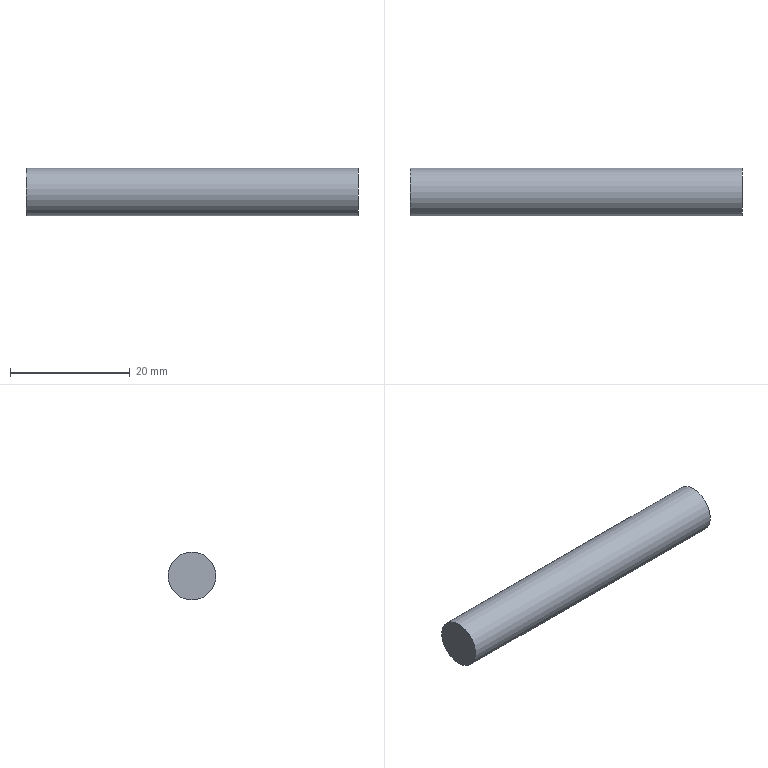Part | STEP file | solid 85 | 1 solid | 3 faces | box 55.5 x 8 x 8 mm | volume 2790 mm3 | plane 2 | cylinder 1 | commonest cylinder face diameters 8 x1